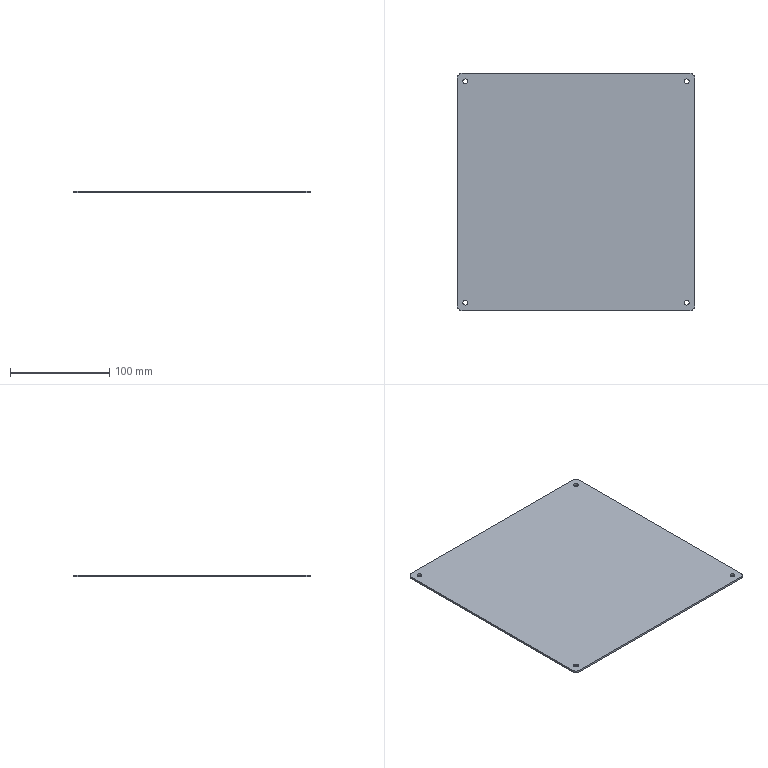Part | STEP file | Panel | 1 solid | 36 faces | box 240 x 240 x 2 mm | volume 114123 mm3 | cylinder 20 | plane 16 | commonest cylinder face diameters 5 x8 10 x4 16 x4 20 x4